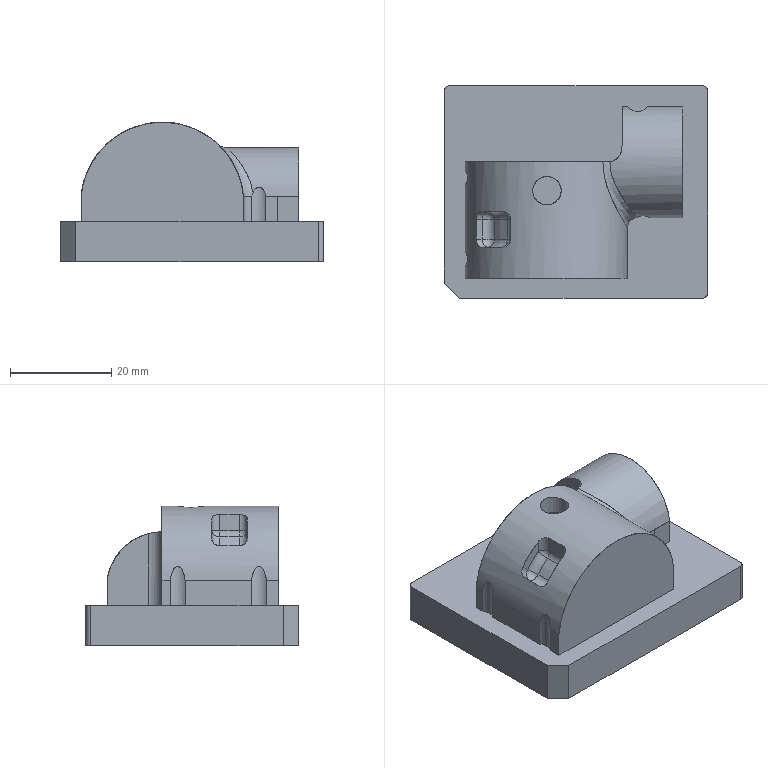NC program | PowerMill | posted with a generic post | part box 52 x 42 x 27.622 mm
Lines 8143 to 8962 of 322299:
N8240 M6
N8241 S18000 M03
N8242 G00 G90 X0.0 Y0.0
N8243 G43 Z9.8022 H2
N8244
N8245 G05 P10000 R4
N8246 X-6.3185 Y-0.295
N8247 Z1.094
N8248 G01 Z-0.106 F3600.0
N8249 X-6.1035 Y-0.4612 Z-0.1107
N8250 X-5.8594 Y-0.544 Z-0.1152
N8251 X-5.6177 Y-0.5434 Z-0.1194
N8252 X-5.3795 Y-0.4612 Z-0.1238
N8253 X-5.1466 Y-0.2884 Z-0.1289
N8254 X-4.9437 Y0.0166 Z-0.1353
N8255 X-4.9417 Y0.0192
N8256 X-4.8637 Y0.1128 Z-0.1375
N8257 X-4.8243 Y0.2159 Z-0.1394
N8258 X-4.8565 Y0.3215 Z-0.1413
N8259 X-5.0027 Y0.5232 Z-0.1457
N8260 X-5.1466 Y0.7219 Z-0.1499
N8261 X-5.3095 Y0.8566 Z-0.1536
N8262 X-5.6187 Y0.9769 Z-0.1594
N8263 X-5.7999 Y0.9831 Z-0.1626
N8264 X-6.0582 Y0.9113 Z-0.1673
N8265 X-6.1121 Y0.8853 Z-0.1683
N8266 X-6.3294 Y0.7285 Z-0.173
N8267 X-6.4172 Y0.6071 Z-0.1756
N8268 X-6.5403 Y0.2704 Z-0.1819
N8269 X-6.5423 Y0.1597 Z-0.1838
N8270 X-6.4711 Y-0.0603 Z-0.1878
N8271 X-6.3685 Y-0.24 Z-0.1914
N8272 X-6.3249 Y-0.2901 Z-0.1926
N8273 X-6.1035 Y-0.4612 Z-0.1975
N8274 X-5.8594 Y-0.544 Z-0.202
N8275 X-5.6177 Y-0.5434 Z-0.2062
N8276 X-5.3795 Y-0.4612 Z-0.2106
N8277 X-5.1466 Y-0.2884 Z-0.2157
N8278 X-4.9437 Y0.0166 Z-0.222
N8279 X-4.9417 Y0.0192 Z-0.2221
N8280 X-4.8637 Y0.1128 Z-0.2242
N8281 X-4.8243 Y0.2159 Z-0.2262
N8282 X-4.8565 Y0.3215 Z-0.2281
N8283 X-5.0027 Y0.5232 Z-0.2324
N8284 X-5.1466 Y0.7219 Z-0.2367
N8285 X-5.3095 Y0.8566 Z-0.2404
N8286 X-5.6187 Y0.9769 Z-0.2462
N8287 X-5.7999 Y0.9831 Z-0.2494
N8288 X-6.0582 Y0.9113 Z-0.254
N8289 X-6.1121 Y0.8853 Z-0.2551
N8290 X-6.3294 Y0.7285 Z-0.2598
N8291 X-6.4172 Y0.6071 Z-0.2624
N8292 X-6.5403 Y0.2704 Z-0.2686
N8293 X-6.5423 Y0.1597 Z-0.2706
N8294 X-6.4711 Y-0.0603 Z-0.2746
N8295 X-6.3685 Y-0.24 Z-0.2782
N8296 X-6.3249 Y-0.2901 Z-0.2794
N8297 X-6.1035 Y-0.4612 Z-0.2843
N8298 X-5.8594 Y-0.544 Z-0.2887
N8299 X-5.6177 Y-0.5434 Z-0.293
N8300 X-5.3795 Y-0.4612 Z-0.2974
N8301 X-5.1466 Y-0.2884 Z-0.3024
N8302 X-4.9437 Y0.0166 Z-0.3088
N8303 X-4.9417 Y0.0192 Z-0.3089
N8304 X-4.8637 Y0.1128 Z-0.311
N8305 X-4.8243 Y0.2159 Z-0.3129
N8306 X-4.8565 Y0.3215 Z-0.3149
N8307 X-5.0027 Y0.5232 Z-0.3192
N8308 X-5.1466 Y0.7219 Z-0.3235
N8309 X-5.3095 Y0.8566 Z-0.3272
N8310 X-5.6187 Y0.9769 Z-0.333
N8311 X-5.7999 Y0.9831 Z-0.3361
N8312 X-6.0582 Y0.9113 Z-0.3408
N8313 X-6.1121 Y0.8853 Z-0.3418
N8314 X-6.3294 Y0.7285 Z-0.3465
N8315 X-6.4172 Y0.6071 Z-0.3491
N8316 X-6.5403 Y0.2704 Z-0.3554
N8317 X-6.5423 Y0.1597 Z-0.3573
N8318 X-6.4711 Y-0.0603 Z-0.3614
N8319 X-6.3685 Y-0.24 Z-0.365
N8320 X-6.3249 Y-0.2901 Z-0.3661
N8321 X-6.1035 Y-0.4612 Z-0.371
N8322 X-5.8594 Y-0.544 Z-0.3755
N8323 X-5.6177 Y-0.5434 Z-0.3797
N8324 X-5.3795 Y-0.4612 Z-0.3841
N8325 X-5.1466 Y-0.2884 Z-0.3892
N8326 X-4.9437 Y0.0166 Z-0.3956
N8327 X-4.9417 Y0.0192
N8328 X-4.8637 Y0.1128 Z-0.3978
N8329 X-4.8243 Y0.2159 Z-0.3997
N8330 X-4.8565 Y0.3215 Z-0.4016
N8331 X-5.0027 Y0.5232 Z-0.406
N8332 X-4.9784 Y0.5408
N8333 X-5.1246 Y0.7426 F6000.0
N8334 X-5.2942 Y0.8828
N8335 X-5.6126 Y1.0067
N8336 X-5.8035 Y1.0133
N8337 X-6.0662 Y0.9402
N8338 X-6.0993 Y0.9277
N8339 X-6.1296 Y0.9097
N8340 X-6.3509 Y0.75
N8341 X-6.444 Y0.6214
N8342 X-6.5685 Y0.2807
N8343 X-6.5806 Y0.2158
N8344 X-6.5709 Y0.1505
N8345 X-6.4987 Y-0.0725
N8346 X-6.3945 Y-0.2548
N8347 X-6.3718 Y-0.2869
N8348 X-6.3432 Y-0.3138
N8349 X-6.1178 Y-0.4881
N8350 X-5.8643 Y-0.574
N8351 X-5.6126 Y-0.5734
N8352 X-5.3654 Y-0.4881
N8353 X-5.1246 Y-0.3094
N8354 X-4.9187 Y0.0
N8355 X-4.8406 Y0.0936
N8356 G03 X-4.8322 Y0.339 I-0.1536 J0.1281
N8357 G01 X-4.9784 Y0.5408
N8358 X-6.5144 Y0.1463 Z-0.3039
N8359 X-6.5153 Y0.1218 Z-0.3044 F3600.0
N8360 X-6.4487 Y-0.0997 Z-0.3084
N8361 X-6.3685 Y-0.24 Z-0.3112
N8362 X-6.3337 Y-0.2828 Z-0.3122
N8363 X-6.1034 Y-0.4613 Z-0.3173
N8364 X-5.8594 Y-0.544 Z-0.3218
N8365 X-5.6177 Y-0.5434 Z-0.326
N8366 X-5.3796 Y-0.4612 Z-0.3304
N8367 X-5.1466 Y-0.2871 Z-0.3355
N8368 X-5.0895 Y-0.2026 Z-0.3372
N8369 X-5.052 Y-0.1463 Z-0.3384
N8370 X-4.991 Y0.0075 Z-0.3413
N8371 X-4.9617 Y0.2455 Z-0.3455
N8372 X-5.007 Y0.4774 Z-0.3496
N8373 X-5.0273 Y0.5125 Z-0.3503
N8374 X-5.133 Y0.6949 Z-0.354
N8375 X-5.1706 Y0.7397 Z-0.355
N8376 X-5.3092 Y0.8563 Z-0.3582
N8377 X-5.6187 Y0.9769 Z-0.364
N8378 X-5.7999 Y0.9831 Z-0.3671
N8379 X-6.0582 Y0.9113 Z-0.3718
N8380 X-6.1121 Y0.8853 Z-0.3729
N8381 X-6.3295 Y0.7285 Z-0.3775
N8382 X-6.4172 Y0.607 Z-0.3802
N8383 X-6.4282 Y0.5771 Z-0.3807
N8384 X-6.507 Y0.3617 Z-0.3847
N8385 X-6.5153 Y0.1218 Z-0.3889
N8386 X-6.4487 Y-0.0997 Z-0.3929
N8387 X-6.3685 Y-0.24 Z-0.3958
N8388 X-6.3337 Y-0.2828 Z-0.3967
N8389 X-6.1034 Y-0.4613 Z-0.4018
N8390 X-5.8594 Y-0.544 Z-0.4063
N8391 X-5.6177 Y-0.5434 Z-0.4105
N8392 X-5.3796 Y-0.4612 Z-0.4149
N8393 X-5.1466 Y-0.2871 Z-0.42
N8394 X-5.0895 Y-0.2026 Z-0.4218
N8395 X-5.052 Y-0.1463 Z-0.423
N8396 X-4.991 Y0.0075 Z-0.4258
N8397 X-4.9617 Y0.2455 Z-0.43
N8398 X-5.007 Y0.4774 Z-0.4342
N8399 X-5.0273 Y0.5125 Z-0.4349
N8400 X-5.133 Y0.6949 Z-0.4385
N8401 X-5.1706 Y0.7397 Z-0.4396
N8402 X-5.3092 Y0.8563 Z-0.4427
N8403 X-5.6187 Y0.9769 Z-0.4485
N8404 X-5.7999 Y0.9831 Z-0.4517
N8405 X-6.0582 Y0.9113 Z-0.4564
N8406 X-6.1121 Y0.8853 Z-0.4574
N8407 X-6.3295 Y0.7285 Z-0.4621
N8408 X-6.4172 Y0.607 Z-0.4647
N8409 X-6.4282 Y0.5771 Z-0.4653
N8410 X-6.507 Y0.3617 Z-0.4693
N8411 X-6.5153 Y0.1218 Z-0.4734
N8412 X-6.4487 Y-0.0997 Z-0.4775
N8413 X-6.3685 Y-0.24 Z-0.4803
N8414 X-6.3337 Y-0.2828 Z-0.4813
N8415 X-6.1034 Y-0.4613 Z-0.4863
N8416 X-5.8594 Y-0.544 Z-0.4908
N8417 X-5.6177 Y-0.5434 Z-0.4951
N8418 X-5.3796 Y-0.4612 Z-0.4995
N8419 X-5.1466 Y-0.2871 Z-0.5045
N8420 X-5.0895 Y-0.2026 Z-0.5063
N8421 X-5.052 Y-0.1463 Z-0.5075
N8422 X-4.991 Y0.0075 Z-0.5104
N8423 X-4.9617 Y0.2455 Z-0.5146
N8424 X-5.007 Y0.4774 Z-0.5187
N8425 X-5.0273 Y0.5125 Z-0.5194
N8426 X-5.133 Y0.6949 Z-0.5231
N8427 X-5.1706 Y0.7397 Z-0.5241
N8428 X-5.3092 Y0.8563 Z-0.5273
N8429 X-5.6187 Y0.9769 Z-0.5331
N8430 X-5.7999 Y0.9831 Z-0.5362
N8431 X-6.0582 Y0.9113 Z-0.5409
N8432 X-6.1121 Y0.8853 Z-0.5419
N8433 X-6.3295 Y0.7285 Z-0.5466
N8434 X-6.4172 Y0.607 Z-0.5492
N8435 X-6.4282 Y0.5771 Z-0.5498
N8436 X-6.507 Y0.3617 Z-0.5538
N8437 X-6.5153 Y0.1218 Z-0.558
N8438 X-6.4487 Y-0.0997 Z-0.562
N8439 X-6.3685 Y-0.24 Z-0.5648
N8440 X-6.3337 Y-0.2828 Z-0.5658
N8441 X-6.1034 Y-0.4613 Z-0.5709
N8442 X-5.8594 Y-0.544 Z-0.5754
N8443 X-5.6177 Y-0.5434 Z-0.5796
N8444 X-5.3796 Y-0.4612 Z-0.584
N8445 X-5.1466 Y-0.2871 Z-0.5891
N8446 X-5.0895 Y-0.2026 Z-0.5909
N8447 X-5.052 Y-0.1463 Z-0.592
N8448 X-4.991 Y0.0075 Z-0.5949
N8449 X-4.9617 Y0.2455 Z-0.5991
N8450 X-5.007 Y0.4774 Z-0.6032
N8451 X-5.0273 Y0.5125 Z-0.6039
N8452 X-5.0014 Y0.5275
N8453 X-5.107 Y0.7099 F6000.0
N8454 X-5.1269 Y0.7382
N8455 X-5.1513 Y0.7627
N8456 X-5.2937 Y0.8824
N8457 X-5.6126 Y1.0067
N8458 X-5.8035 Y1.0133
N8459 X-6.0662 Y0.9402
N8460 X-6.0993 Y0.9277
N8461 X-6.1296 Y0.9097
N8462 X-6.351 Y0.75
N8463 X-6.4439 Y0.6212
N8464 X-6.4564 Y0.5875
N8465 X-6.5368 Y0.3675
N8466 X-6.5454 Y0.1179
N8467 X-6.4764 Y-0.1117
N8468 X-6.3946 Y-0.2549
N8469 X-6.3758 Y-0.2821
N8470 X-6.3528 Y-0.306
N8471 X-6.1178 Y-0.4881
N8472 X-5.8643 Y-0.574
N8473 X-5.6126 Y-0.5733
N8474 X-5.3654 Y-0.4881
N8475 X-5.1246 Y-0.3081
N8476 X-5.0646 Y-0.2193
N8477 X-5.0253 Y-0.1603
N8478 X-4.9617 Y0.0
N8479 X-4.9313 Y0.2466
N8480 X-4.9785 Y0.4881
N8481 X-5.0014 Y0.5275
N8482 X-6.512 Y0.1596 Z-0.5019
N8483 X-6.5133 Y0.1228 Z-0.5026 F3600.0
N8484 X-6.446 Y-0.1046 Z-0.5067
N8485 X-6.3687 Y-0.2398 Z-0.5094
N8486 X-6.3581 Y-0.2561 Z-0.5098
N8487 X-6.3439 Y-0.2731 Z-0.5101
N8488 X-6.1034 Y-0.4613 Z-0.5155
N8489 X-5.8594 Y-0.544 Z-0.52
N8490 X-5.6177 Y-0.5433 Z-0.5242
N8491 X-5.3796 Y-0.4612 Z-0.5286
N8492 X-5.1466 Y-0.2859 Z-0.5337
N8493 X-5.0538 Y-0.1478 Z-0.5366
N8494 X-4.9929 Y0.0075 Z-0.5395
N8495 X-4.963 Y0.2456 Z-0.5437
N8496 X-5.0094 Y0.4774 Z-0.5478
N8497 X-5.0291 Y0.5116 Z-0.5485
N8498 X-5.1448 Y0.7126 Z-0.5525
N8499 X-5.1526 Y0.7222 Z-0.5528
N8500 X-5.3089 Y0.856 Z-0.5563
N8501 X-5.6187 Y0.9769 Z-0.5621
N8502 X-5.7999 Y0.9831 Z-0.5653
N8503 X-6.0583 Y0.9112 Z-0.57
N8504 X-6.1121 Y0.8854 Z-0.571
N8505 X-6.1338 Y0.8697 Z-0.5715
N8506 X-6.3267 Y0.7305 Z-0.5757
N8507 X-6.4144 Y0.6104 Z-0.5782
N8508 X-6.5041 Y0.3665 Z-0.5828
N8509 X-6.5133 Y0.1228 Z-0.587
N8510 X-6.446 Y-0.1046 Z-0.5912
N8511 X-6.3687 Y-0.2398 Z-0.5939
N8512 X-6.3581 Y-0.2561 Z-0.5942
N8513 X-6.3439 Y-0.2731 Z-0.5946
N8514 X-6.1034 Y-0.4613 Z-0.6
N8515 X-5.8594 Y-0.544 Z-0.6044
N8516 X-5.6177 Y-0.5433 Z-0.6087
N8517 X-5.3796 Y-0.4612 Z-0.6131
N8518 X-5.1466 Y-0.2859 Z-0.6181
N8519 X-5.0538 Y-0.1478 Z-0.6211
N8520 X-4.9929 Y0.0075 Z-0.624
N8521 X-4.963 Y0.2456 Z-0.6282
N8522 X-5.0094 Y0.4774 Z-0.6323
N8523 X-5.0291 Y0.5116 Z-0.633
N8524 X-5.1448 Y0.7126 Z-0.637
N8525 X-5.1526 Y0.7222 Z-0.6372
N8526 X-5.3089 Y0.856 Z-0.6408
N8527 X-5.6187 Y0.9769 Z-0.6466
N8528 X-5.7999 Y0.9831 Z-0.6498
N8529 X-6.0583 Y0.9112 Z-0.6545
N8530 X-6.1121 Y0.8854 Z-0.6555
N8531 X-6.1338 Y0.8697 Z-0.656
N8532 X-6.3267 Y0.7305 Z-0.6601
N8533 X-6.4144 Y0.6104 Z-0.6627
N8534 X-6.5041 Y0.3665 Z-0.6673
N8535 X-6.5133 Y0.1228 Z-0.6715
N8536 X-6.446 Y-0.1046 Z-0.6757
N8537 X-6.3687 Y-0.2398 Z-0.6784
N8538 X-6.3581 Y-0.2561 Z-0.6787
N8539 X-6.3439 Y-0.2731 Z-0.6791
N8540 X-6.1034 Y-0.4613 Z-0.6844
N8541 X-5.8594 Y-0.544 Z-0.6889
N8542 X-5.6177 Y-0.5433 Z-0.6931
N8543 X-5.3796 Y-0.4612 Z-0.6975
N8544 X-5.1466 Y-0.2859 Z-0.7026
N8545 X-5.0538 Y-0.1478 Z-0.7055
N8546 X-4.9929 Y0.0075 Z-0.7084
N8547 X-4.963 Y0.2456 Z-0.7126
N8548 X-5.0094 Y0.4774 Z-0.7168
N8549 X-5.0291 Y0.5116 Z-0.7174
N8550 X-5.1448 Y0.7126 Z-0.7215
N8551 X-5.1526 Y0.7222 Z-0.7217
N8552 X-5.3089 Y0.856 Z-0.7253
N8553 X-5.6187 Y0.9769 Z-0.7311
N8554 X-5.7999 Y0.9831 Z-0.7343
N8555 X-6.0583 Y0.9112 Z-0.7389
N8556 X-6.1121 Y0.8854 Z-0.74
N8557 X-6.1338 Y0.8697 Z-0.7405
N8558 X-6.3267 Y0.7305 Z-0.7446
N8559 X-6.4144 Y0.6104 Z-0.7472
N8560 X-6.5041 Y0.3665 Z-0.7517
N8561 X-6.5133 Y0.1228 Z-0.756
N8562 X-6.446 Y-0.1046 Z-0.7601
N8563 X-6.3687 Y-0.2398 Z-0.7628
N8564 X-6.3581 Y-0.2561 Z-0.7632
N8565 X-6.3439 Y-0.2731 Z-0.7636
N8566 X-6.1034 Y-0.4613 Z-0.7689
N8567 X-5.8594 Y-0.544 Z-0.7734
N8568 X-5.6177 Y-0.5433 Z-0.7776
N8569 X-5.3796 Y-0.4612 Z-0.782
N8570 X-5.1466 Y-0.2859 Z-0.7871
N8571 X-5.0538 Y-0.1478 Z-0.79
N8572 X-4.9929 Y0.0075 Z-0.7929
N8573 X-4.963 Y0.2456 Z-0.7971
N8574 X-5.0094 Y0.4774 Z-0.8012
N8575 X-5.0291 Y0.5116 Z-0.8019
N8576 X-5.0031 Y0.5265
N8577 X-5.1197 Y0.7292 F6000.0
N8578 X-5.1254 Y0.7366
N8579 X-5.1316 Y0.7437
N8580 X-5.2932 Y0.8821
N8581 X-5.6126 Y1.0067
N8582 X-5.8035 Y1.0133
N8583 X-6.0663 Y0.9401
N8584 X-6.0993 Y0.9277
N8585 X-6.1296 Y0.9097
N8586 X-6.1514 Y0.894
N8587 X-6.3481 Y0.7521
N8588 X-6.4411 Y0.6247
N8589 X-6.5339 Y0.3724
N8590 X-6.5435 Y0.119
N8591 X-6.4737 Y-0.1165
N8592 X-6.3946 Y-0.2549
N8593 X-6.3945 Y-0.2551
N8594 X-6.3943 Y-0.2554
N8595 X-6.3829 Y-0.2731
N8596 X-6.3738 Y-0.2846
N8597 X-6.364 Y-0.2955
N8598 X-6.1178 Y-0.4881
N8599 X-5.8643 Y-0.574
N8600 X-5.6126 Y-0.5733
N8601 X-5.3654 Y-0.4881
N8602 X-5.1246 Y-0.3069
N8603 X-5.027 Y-0.1618
N8604 X-4.9636 Y0.0
N8605 X-4.9327 Y0.2467
N8606 X-4.981 Y0.4881
N8607 X-5.0031 Y0.5265
N8608 X-6.5092 Y0.1785 Z-0.6999
N8609 X-6.5112 Y0.1225 Z-0.7009 F3600.0
N8610 X-6.4422 Y-0.1113 Z-0.7051
N8611 X-6.3836 Y-0.2139 Z-0.7072
N8612 X-6.3483 Y-0.2679 Z-0.7083
N8613 X-6.1033 Y-0.4613 Z-0.7138
N8614 X-5.8594 Y-0.544 Z-0.7183
N8615 X-5.6177 Y-0.5433 Z-0.7225
N8616 X-5.3797 Y-0.4613 Z-0.7269
N8617 X-5.1467 Y-0.2835 Z-0.732
N8618 X-5.0545 Y-0.146 Z-0.7349
N8619 X-4.9947 Y0.0074 Z-0.7377
N8620 X-4.9646 Y0.2454 Z-0.7419
N8621 X-5.0118 Y0.4773 Z-0.7461
N8622 X-5.0308 Y0.5106 Z-0.7467
N8623 X-5.1481 Y0.7154 Z-0.7508
N8624 X-5.3084 Y0.8555 Z-0.7546
N8625 X-5.6188 Y0.9769 Z-0.7604
N8626 X-5.7999 Y0.9831 Z-0.7635
N8627 X-6.0583 Y0.9112 Z-0.7682
N8628 X-6.112 Y0.8854 Z-0.7693
N8629 X-6.1642 Y0.8479 Z-0.7704
N8630 X-6.3259 Y0.7312 Z-0.7739
N8631 X-6.413 Y0.6109 Z-0.7765
N8632 X-6.5023 Y0.3664 Z-0.781
N8633 X-6.5112 Y0.1225 Z-0.7853
N8634 X-6.4422 Y-0.1113 Z-0.7895
N8635 X-6.3836 Y-0.2139 Z-0.7916
N8636 X-6.3483 Y-0.2679 Z-0.7927
N8637 X-6.1033 Y-0.4613 Z-0.7981
N8638 X-5.8594 Y-0.544 Z-0.8026
N8639 X-5.6177 Y-0.5433 Z-0.8069
N8640 X-5.3797 Y-0.4613 Z-0.8113
N8641 X-5.1467 Y-0.2835 Z-0.8164
N8642 X-5.0545 Y-0.146 Z-0.8193
N8643 X-4.9947 Y0.0074 Z-0.8221
N8644 X-4.9646 Y0.2454 Z-0.8263
N8645 X-5.0118 Y0.4773 Z-0.8304
N8646 X-5.0308 Y0.5106 Z-0.8311
N8647 X-5.1481 Y0.7154 Z-0.8352
N8648 X-5.3084 Y0.8555 Z-0.8389
N8649 X-5.6188 Y0.9769 Z-0.8448
N8650 X-5.7999 Y0.9831 Z-0.8479
N8651 X-6.0583 Y0.9112 Z-0.8526
N8652 X-6.112 Y0.8854 Z-0.8536
N8653 X-6.1642 Y0.8479 Z-0.8548
N8654 X-6.3259 Y0.7312 Z-0.8583
N8655 X-6.413 Y0.6109 Z-0.8608
N8656 X-6.5023 Y0.3664 Z-0.8654
N8657 X-6.5112 Y0.1225 Z-0.8696
N8658 X-6.4422 Y-0.1113 Z-0.8739
N8659 X-6.3836 Y-0.2139 Z-0.876
N8660 X-6.3483 Y-0.2679 Z-0.8771
N8661 X-6.1033 Y-0.4613 Z-0.8825
N8662 X-5.8594 Y-0.544 Z-0.887
N8663 X-5.6177 Y-0.5433 Z-0.8912
N8664 X-5.3797 Y-0.4613 Z-0.8956
N8665 X-5.1467 Y-0.2835 Z-0.9008
N8666 X-5.0545 Y-0.146 Z-0.9036
N8667 X-4.9947 Y0.0074 Z-0.9065
N8668 X-4.9646 Y0.2454 Z-0.9107
N8669 X-5.0118 Y0.4773 Z-0.9148
N8670 X-5.0308 Y0.5106 Z-0.9155
N8671 X-5.1481 Y0.7154 Z-0.9196
N8672 X-5.3084 Y0.8555 Z-0.9233
N8673 X-5.6188 Y0.9769 Z-0.9292
N8674 X-5.7999 Y0.9831 Z-0.9323
N8675 X-6.0583 Y0.9112 Z-0.937
N8676 X-6.112 Y0.8854 Z-0.938
N8677 X-6.1642 Y0.8479 Z-0.9392
N8678 X-6.3259 Y0.7312 Z-0.9426
N8679 X-6.413 Y0.6109 Z-0.9452
N8680 X-6.5023 Y0.3664 Z-0.9498
N8681 X-6.5112 Y0.1225 Z-0.954
N8682 X-6.4422 Y-0.1113 Z-0.9583
N8683 X-6.3836 Y-0.2139 Z-0.9603
N8684 X-6.3483 Y-0.2679 Z-0.9615
N8685 X-6.1033 Y-0.4613 Z-0.9669
N8686 X-5.8594 Y-0.544 Z-0.9714
N8687 X-5.6177 Y-0.5433 Z-0.9756
N8688 X-5.3797 Y-0.4613 Z-0.98
N8689 X-5.1467 Y-0.2835 Z-0.9851
N8690 X-5.0545 Y-0.146 Z-0.988
N8691 X-4.9947 Y0.0074 Z-0.9909
N8692 X-4.9646 Y0.2454 Z-0.9951
N8693 X-5.0118 Y0.4773 Z-0.9992
N8694 X-5.0308 Y0.5106 Z-0.9999
N8695 X-5.0048 Y0.5255
N8696 X-5.1246 Y0.7347 F6000.0
N8697 X-5.2926 Y0.8816
N8698 X-5.6126 Y1.0067
N8699 X-5.8035 Y1.0133
N8700 X-6.0663 Y0.9401
N8701 X-6.0993 Y0.9277
N8702 X-6.1296 Y0.9098
N8703 X-6.1817 Y0.8722
N8704 X-6.3474 Y0.7527
N8705 X-6.4397 Y0.6251
N8706 X-6.5321 Y0.3723
N8707 X-6.5414 Y0.1187
N8708 X-6.47 Y-0.1231
N8709 X-6.4092 Y-0.2295
N8710 X-6.3711 Y-0.2879
N8711 X-6.3707 Y-0.2883
N8712 X-6.3703 Y-0.2888
N8713 X-6.1178 Y-0.4881
N8714 X-5.8643 Y-0.574
N8715 X-5.6126 Y-0.5733
N8716 X-5.3654 Y-0.4881
N8717 X-5.1246 Y-0.3043
N8718 X-5.0278 Y-0.16
N8719 X-4.9654 Y0.0
N8720 X-4.9342 Y0.2465
N8721 X-4.9833 Y0.4881
N8722 X-5.0048 Y0.5255
N8723 X-6.506 Y0.2162 Z-0.8979
N8724 X-6.509 Y0.1214 Z-0.8995 F3600.0
N8725 X-6.4372 Y-0.1201 Z-0.9039
N8726 X-6.4014 Y-0.1828 Z-0.9052
N8727 X-6.3454 Y-0.2678 Z-0.907
N8728 X-6.1265 Y-0.4427 Z-0.9118
N8729 X-6.0749 Y-0.4709 Z-0.9129
N8730 X-5.8594 Y-0.544 Z-0.9168
N8731 X-5.6177 Y-0.5433 Z-0.9211
N8732 X-5.3799 Y-0.4613 Z-0.9255
N8733 X-5.1468 Y-0.28 Z-0.9306
N8734 X-5.0562 Y-0.1439 Z-0.9335
N8735 X-4.9966 Y0.0075 Z-0.9363
N8736 X-4.9657 Y0.2451 Z-0.9405
N8737 X-5.014 Y0.4773 Z-0.9446
N8738 X-5.0325 Y0.5097 Z-0.9453
N8739 X-5.1482 Y0.7125 Z-0.9493
N8740 X-5.3086 Y0.8556 Z-0.9531
N8741 X-5.6186 Y0.9769 Z-0.9589
N8742 X-5.7999 Y0.9831 Z-0.9621
N8743 X-6.0574 Y0.9115 Z-0.9667
N8744 X-6.1124 Y0.8847 Z-0.9678
N8745 X-6.2967 Y0.7495 Z-0.9718
N8746 X-6.3422 Y0.6993 Z-0.973
N8747 X-6.4422 Y0.531 Z-0.9764
N8748 X-6.4991 Y0.3751 Z-0.9793
N8749 X-6.5013 Y0.3662 Z-0.9794
N8750 X-6.509 Y0.1214 Z-0.9837
N8751 X-6.4372 Y-0.1201 Z-0.9881
N8752 X-6.4014 Y-0.1828 Z-0.9894
N8753 X-6.3454 Y-0.2678 Z-0.9912
N8754 X-6.1265 Y-0.4427 Z-0.996
N8755 X-6.0749 Y-0.4709 Z-0.9971
N8756 X-5.8594 Y-0.544 Z-1.001
N8757 X-5.6177 Y-0.5433 Z-1.0053
N8758 X-5.3799 Y-0.4613 Z-1.0097
N8759 X-5.1468 Y-0.28 Z-1.0148
N8760 X-5.0562 Y-0.1439 Z-1.0177
N8761 X-4.9966 Y0.0075 Z-1.0205
N8762 X-4.9657 Y0.2451 Z-1.0247
N8763 X-5.014 Y0.4773 Z-1.0288
N8764 X-5.0325 Y0.5097 Z-1.0295
N8765 X-5.1482 Y0.7125 Z-1.0335
N8766 X-5.3086 Y0.8556 Z-1.0373
N8767 X-5.6186 Y0.9769 Z-1.0431
N8768 X-5.7999 Y0.9831 Z-1.0463
N8769 X-6.0574 Y0.9115 Z-1.0509
N8770 X-6.1124 Y0.8847 Z-1.052
N8771 X-6.2967 Y0.7495 Z-1.056
N8772 X-6.3422 Y0.6993 Z-1.0572
N8773 X-6.4422 Y0.531 Z-1.0606
N8774 X-6.4991 Y0.3751 Z-1.0635
N8775 X-6.5013 Y0.3662 Z-1.0636
N8776 X-6.509 Y0.1214 Z-1.0679
N8777 X-6.4372 Y-0.1201 Z-1.0723
N8778 X-6.4014 Y-0.1828 Z-1.0736
N8779 X-6.3454 Y-0.2678 Z-1.0754
N8780 X-6.1265 Y-0.4427 Z-1.0802
N8781 X-6.0749 Y-0.4709 Z-1.0813
N8782 X-5.8594 Y-0.544 Z-1.0852
N8783 X-5.6177 Y-0.5433 Z-1.0895
N8784 X-5.3799 Y-0.4613 Z-1.0939
N8785 X-5.1468 Y-0.28 Z-1.099
N8786 X-5.0562 Y-0.1439 Z-1.1019
N8787 X-4.9966 Y0.0075 Z-1.1047
N8788 X-4.9657 Y0.2451 Z-1.1089
N8789 X-5.014 Y0.4773 Z-1.113
N8790 X-5.0325 Y0.5097 Z-1.1137
N8791 X-5.1482 Y0.7125 Z-1.1177
N8792 X-5.3086 Y0.8556 Z-1.1215
N8793 X-5.6186 Y0.9769 Z-1.1273
N8794 X-5.7999 Y0.9831 Z-1.1305
N8795 X-6.0574 Y0.9115 Z-1.1351
N8796 X-6.1124 Y0.8847 Z-1.1362
N8797 X-6.2967 Y0.7495 Z-1.1402
N8798 X-6.3422 Y0.6993 Z-1.1414
N8799 X-6.4422 Y0.531 Z-1.1448
N8800 X-6.4991 Y0.3751 Z-1.1477
N8801 X-6.5013 Y0.3662 Z-1.1478
N8802 X-6.509 Y0.1214 Z-1.1521
N8803 X-6.4372 Y-0.1201 Z-1.1565
N8804 X-6.4014 Y-0.1828 Z-1.1578
N8805 X-6.3454 Y-0.2678 Z-1.1596
N8806 X-6.1265 Y-0.4427 Z-1.1644
N8807 X-6.0749 Y-0.4709 Z-1.1655
N8808 X-5.8594 Y-0.544 Z-1.1694
N8809 X-5.6177 Y-0.5433 Z-1.1737
N8810 X-5.3799 Y-0.4613 Z-1.1781
N8811 X-5.1468 Y-0.28 Z-1.1832
N8812 X-5.0562 Y-0.1439 Z-1.1861
N8813 X-4.9966 Y0.0075 Z-1.1889
N8814 X-4.9657 Y0.2451 Z-1.1931
N8815 X-5.014 Y0.4773 Z-1.1972
N8816 X-5.0325 Y0.5097 Z-1.1979
N8817 X-5.0064 Y0.5246
N8818 X-5.1246 Y0.7317 F6000.0
N8819 X-5.292 Y0.881
N8820 X-5.2941 Y0.8822
N8821 X-5.6117 Y1.0064
N8822 X-5.6126 Y1.0067
N8823 X-5.8035 Y1.0133
N8824 X-6.0654 Y0.9404
N8825 X-6.0992 Y0.9276
N8826 X-6.1301 Y0.9089
N8827 X-6.3144 Y0.7737
N8828 X-6.3442 Y0.7468
N8829 X-6.368 Y0.7146
N8830 X-6.4694 Y0.544
N8831 X-6.5279 Y0.3839
N8832 X-6.5312 Y0.3703
N8833 X-6.5391 Y0.1175
N8834 X-6.465 Y-0.132
N8835 X-6.4269 Y-0.1985
N8836 X-6.3678 Y-0.2883
N8837 X-6.1452 Y-0.4662
N8838 X-6.1163 Y-0.4854
N8839 X-6.0846 Y-0.4993
N8840 X-5.8643 Y-0.574
N8841 X-5.6126 Y-0.5733
N8842 X-5.3654 Y-0.4881
N8843 X-5.1246 Y-0.3007
N8844 X-5.0295 Y-0.1578
N8845 X-4.9673 Y0.0
N8846 X-4.9353 Y0.2462
N8847 X-4.9856 Y0.4881
N8848 X-5.0064 Y0.5246
N8849 X-6.5053 Y0.2407 Z-1.0958
N8850 X-6.5083 Y0.1426 Z-1.0976 F3600.0
N8851 X-6.5073 Y0.1218 Z-1.0979
N8852 X-6.4321 Y-0.1291 Z-1.1025
N8853 X-6.4191 Y-0.1518 Z-1.1029
N8854 X-6.3435 Y-0.267 Z-1.1053
N8855 X-6.1267 Y-0.4423 Z-1.1102
N8856 X-6.0744 Y-0.4711 Z-1.1113
N8857 X-5.8594 Y-0.544 Z-1.1152
N8858 X-5.6177 Y-0.5433 Z-1.1194
N8859 X-5.38 Y-0.4614 Z-1.1238
N8860 X-5.1469 Y-0.2766 Z-1.129
N8861 X-5.0576 Y-0.1419 Z-1.1318
N8862 X-4.9984 Y0.0076 Z-1.1346
N8863 X-4.9663 Y0.2452 Z-1.1388
N8864 X-5.0156 Y0.4773 Z-1.143
N8865 X-5.0337 Y0.509 Z-1.1436
N8866 X-5.1483 Y0.7099 Z-1.1476
N8867 X-5.3087 Y0.8557 Z-1.1514
N8868 X-5.6184 Y0.9769 Z-1.1572
N8869 X-5.7999 Y0.9831 Z-1.1604
N8870 X-6.0564 Y0.9117 Z-1.165
N8871 X-6.1128 Y0.884 Z-1.1661
N8872 X-6.2979 Y0.7452 Z-1.1702
N8873 X-6.342 Y0.6962 Z-1.1713
N8874 X-6.4451 Y0.5233 Z-1.1748
N8875 X-6.4817 Y0.423 Z-1.1767
N8876 X-6.5036 Y0.2952 Z-1.179
N8877 X-6.5083 Y0.1426 Z-1.1816
N8878 X-6.5073 Y0.1218 Z-1.182
N8879 X-6.4321 Y-0.1291 Z-1.1866
N8880 X-6.4191 Y-0.1518 Z-1.187
N8881 X-6.3435 Y-0.267 Z-1.1894
N8882 X-6.1267 Y-0.4423 Z-1.1943
N8883 X-6.0744 Y-0.4711 Z-1.1953
N8884 X-5.8594 Y-0.544 Z-1.1993
N8885 X-5.6177 Y-0.5433 Z-1.2035
N8886 X-5.38 Y-0.4614 Z-1.2079
N8887 X-5.1469 Y-0.2766 Z-1.2131
N8888 X-5.0576 Y-0.1419 Z-1.2159
N8889 X-4.9984 Y0.0076 Z-1.2187
N8890 X-4.9663 Y0.2452 Z-1.2229
N8891 X-5.0156 Y0.4773 Z-1.227
N8892 X-5.0337 Y0.509 Z-1.2277
N8893 X-5.1483 Y0.7099 Z-1.2317
N8894 X-5.3087 Y0.8557 Z-1.2355
N8895 X-5.6184 Y0.9769 Z-1.2413
N8896 X-5.7999 Y0.9831 Z-1.2445
N8897 X-6.0564 Y0.9117 Z-1.2491
N8898 X-6.1128 Y0.884 Z-1.2502
N8899 X-6.2979 Y0.7452 Z-1.2543
N8900 X-6.342 Y0.6962 Z-1.2554
N8901 X-6.4451 Y0.5233 Z-1.2589
N8902 X-6.4817 Y0.423 Z-1.2608
N8903 X-6.5036 Y0.2952 Z-1.263
N8904 X-6.5083 Y0.1426 Z-1.2657
N8905 X-6.5073 Y0.1218 Z-1.2661
N8906 X-6.4321 Y-0.1291 Z-1.2706
N8907 X-6.4191 Y-0.1518 Z-1.2711
N8908 X-6.3435 Y-0.267 Z-1.2735
N8909 X-6.1267 Y-0.4423 Z-1.2784
N8910 X-6.0744 Y-0.4711 Z-1.2794
N8911 X-5.8594 Y-0.544 Z-1.2834
N8912 X-5.6177 Y-0.5433 Z-1.2876
N8913 X-5.38 Y-0.4614 Z-1.292
N8914 X-5.1469 Y-0.2766 Z-1.2972
N8915 X-5.0576 Y-0.1419 Z-1.3
N8916 X-4.9984 Y0.0076 Z-1.3028
N8917 X-4.9663 Y0.2452 Z-1.307
N8918 X-5.0156 Y0.4773 Z-1.3111
N8919 X-5.0337 Y0.509 Z-1.3118
N8920 X-5.1483 Y0.7099 Z-1.3158
N8921 X-5.3087 Y0.8557 Z-1.3196
N8922 X-5.6184 Y0.9769 Z-1.3254
N8923 X-5.7999 Y0.9831 Z-1.3286
N8924 X-6.0564 Y0.9117 Z-1.3332
N8925 X-6.1128 Y0.884 Z-1.3343
N8926 X-6.2979 Y0.7452 Z-1.3383
N8927 X-6.342 Y0.6962 Z-1.3395
N8928 X-6.4451 Y0.5233 Z-1.343
N8929 X-6.4817 Y0.423 Z-1.3449
N8930 X-6.5036 Y0.2952 Z-1.3471
N8931 X-6.5083 Y0.1426 Z-1.3498
N8932 X-6.5073 Y0.1218 Z-1.3502
N8933 X-6.4321 Y-0.1291 Z-1.3547
N8934 X-6.4191 Y-0.1518 Z-1.3552
N8935 X-6.3435 Y-0.267 Z-1.3576
N8936 X-6.1267 Y-0.4423 Z-1.3625
N8937 X-6.0744 Y-0.4711 Z-1.3635
N8938 X-5.8594 Y-0.544 Z-1.3675
N8939 X-5.6177 Y-0.5433 Z-1.3717
N8940 X-5.38 Y-0.4614 Z-1.3761
N8941 X-5.1469 Y-0.2766 Z-1.3813
N8942 X-5.0576 Y-0.1419 Z-1.3841
N8943 X-4.9984 Y0.0076 Z-1.3869
N8944 X-4.9663 Y0.2452 Z-1.3911
N8945 X-5.0156 Y0.4773 Z-1.3952
N8946 X-5.0337 Y0.509 Z-1.3958
N8947 X-5.0077 Y0.5239
N8948 X-5.1246 Y0.7289 F6000.0
N8949 X-5.2914 Y0.8805
N8950 X-5.2954 Y0.8828
N8951 X-5.6108 Y1.0061
N8952 X-5.6126 Y1.0067
N8953 X-5.8035 Y1.0133
N8954 X-6.0644 Y0.9406
N8955 X-6.0991 Y0.9274
N8956 X-6.1308 Y0.908
N8957 X-6.3159 Y0.7692
N8958 X-6.3447 Y0.7429
N8959 X-6.3678 Y0.7116
N8960 X-6.4723 Y0.5362
N8961 X-6.5108 Y0.4308
N8962 X-6.5335 Y0.2982
N8963 X-6.5384 Y0.1423
N8964 X-6.5371 Y0.1166
N8965 X-6.4598 Y-0.1411
N8966 X-6.4447 Y-0.1675
N8967 X-6.366 Y-0.2874
N8968 X-6.1456 Y-0.4656
N8969 X-6.1163 Y-0.4853
N8970 X-6.084 Y-0.4995
N8971 X-5.8643 Y-0.574
N8972 X-5.6126 Y-0.5733
N8973 X-5.3654 Y-0.4881
N8974 X-5.1246 Y-0.2971
N8975 X-5.0309 Y-0.1559
N8976 X-4.9692 Y0.0
N8977 X-4.9359 Y0.2463
N8978 X-4.9872 Y0.4881
N8979 X-5.0077 Y0.5239
N8980 G00 Z3.794
N8981 G01 X-0.4121 Y2.0444 F10000.0
N8982 G00 Z0.794
N8983 G01 Z-0.406 F3600.0
N8984 X-0.4308 Y2.056 F6000.0
N8985 G03 X-0.7033 Y1.9916 I-0.1041 J-0.1685
N8986 G01 X-1.7884 Y0.2347
N8987 X-1.7796 Y0.1558
N8988 X-1.7408 Y0.0865
N8989 X-1.7082 Y0.0485
N8990 X-1.43 Y-0.4881
N8991 X-1.3099 Y-0.9761
N8992 X-1.2985 Y-3.4164
N8993 X-1.3419 Y-11.7133
N8994 X-1.316 Y-13.1774
N8995 X-1.3603 Y-13.6655
N8996 X-1.3776 Y-16.5938
N8997 X-1.3508 Y-17.0818
N8998 X-1.3904 Y-17.5699
N8999 X-1.5603 Y-18.0579
N9000 X-1.7082 Y-18.3037
N9001 X-1.9043 Y-18.546
N9002 X-2.1962 Y-18.7938
N9003 X-2.6497 Y-19.0341
N9004 X-3.1723 Y-19.1533
N9005 X-3.6604 Y-19.1611
N9006 X-8.0529
N9007 X-8.5409 Y-19.1558
N9008 X-9.029 Y-19.06
N9009 X-9.517 Y-18.825
N9010 X-9.8495 Y-18.546
N9011 X-10.0051 Y-18.363
N9012 X-10.1961 Y-18.0579
N9013 X-10.3652 Y-17.5699
N9014 X-10.4058 Y-17.0818
N9015 X-10.3763 Y-16.5938
N9016 Y-14.1535
N9017 X-10.4473 Y-13.1774
N9018 X-10.4431 Y-0.9761
N9019 X-10.4517 Y-0.4881
N9020 X-10.392 Y0.0
N9021 X-10.3463 Y0.1552
N9022 X-10.3383 Y0.2153
N9023 X-10.3486 Y0.2751
N9024 X-10.3795 Y0.3675
N9025 X-10.457 Y0.9761
N9026 X-10.403 Y2.4403
N9027 X-10.4474 Y2.9283
N9028 X-10.4467 Y5.8566
N9029 X-10.406 Y6.3447
N9030 X-10.2375 Y6.8327
N9031 X-10.0051 Y7.1897
N9032 X-9.8925 Y7.3208
N9033 X-9.517 Y7.6288
N9034 X-9.1631 Y7.8088
N9035 X-9.029 Y7.8537
N9036 X-8.5409 Y7.9387
N9037 X-3.6604 Y7.9413
N9038 X-3.1723 Y7.9355
N9039 X-2.6843 Y7.8366
N9040 X-2.1962 Y7.5957
N9041 X-1.8677 Y7.3208
N9042 X-1.5255 Y6.8327
N9043 X-1.357 Y6.3447
N9044 X-1.317 Y5.8566
N9045 X-1.3093 Y1.4642
N9046 X-1.412 Y0.9761
N9047 X-1.6922 Y0.4235
N9048 X-1.6957 Y0.4146
N9049 X-1.7126 Y0.3769
N9050 X-1.741 Y0.347
N9051 X-1.7734 Y0.2945
N9052 X-1.7884 Y0.2347
N9053 X0.6126 Y1.3624 Z-0.6039
N9054 X0.5934 Y1.3732
N9055 G03 X0.3239 Y1.297 I-0.0967 J-0.1728
N9056 G01 X-0.3089 Y0.1659
N9057 X-0.3394 Y-0.4881
N9058 Y-12.6894
N9059 X-0.2992 Y-13.1774